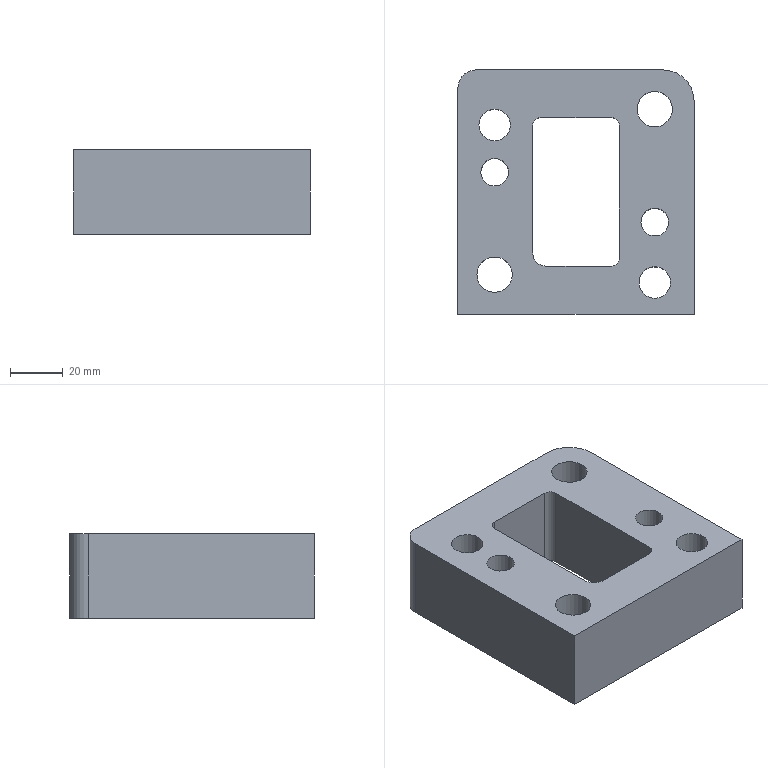Part | STEP file | lll_id3174_x_t | 1 solid | 26 faces | box 90 x 93 x 32 mm | volume 180117 mm3 | cylinder 14 | plane 12 | commonest cylinder face diameters 6 x3 10.505 x2 12 x2 13.509 x2 20.008 x2 10 x1
STEP:
#1=CARTESIAN_POINT('',(926.252,-22.25,60.5));
#2=VERTEX_POINT('',#1);
#3=CARTESIAN_POINT('',(921.,-22.25,60.5));
#4=DIRECTION('',(0.,0.,1.));
#5=DIRECTION('',(1.,0.,0.));
#6=AXIS2_PLACEMENT_3D('',#3,#4,#5);
#7=CIRCLE('',#6,5.253);
#8=EDGE_CURVE('',#2,#2,#7,.T.);
#9=ORIENTED_EDGE('',*,*,#8,.T.);
#10=EDGE_LOOP('',(#9));
#11=FACE_BOUND('',#10,.T.);
#12=CARTESIAN_POINT('',(849.996,-42.25,60.5));
#13=VERTEX_POINT('',#12);
#14=CARTESIAN_POINT('',(860.,-42.25,60.5));
#15=DIRECTION('',(0.,0.,1.));
#16=DIRECTION('',(-1.,0.,0.));
#17=AXIS2_PLACEMENT_3D('',#14,#15,#16);
#18=CIRCLE('',#17,10.004);
#19=EDGE_CURVE('',#13,#13,#18,.T.);
#20=ORIENTED_EDGE('',*,*,#19,.T.);
#21=EDGE_LOOP('',(#20));
#22=FACE_BOUND('',#21,.T.);
#23=CARTESIAN_POINT('',(874.5,14.5,60.5));
#24=VERTEX_POINT('',#23);
#25=CARTESIAN_POINT('',(874.5,-34.,60.5));
#26=VERTEX_POINT('',#25);
#27=CARTESIAN_POINT('',(874.5,0.,60.5));
#28=DIRECTION('',(0.,-1.,0.));
#29=VECTOR('',#28,1.);
#30=LINE('',#27,#29);
#31=EDGE_CURVE('',#24,#26,#30,.T.);
#32=ORIENTED_EDGE('',*,*,#31,.T.);
#33=CARTESIAN_POINT('',(879.5,-39.,60.5));
#34=VERTEX_POINT('',#33);
#35=CARTESIAN_POINT('',(879.5,-34.,60.5));
#36=DIRECTION('',(0.,0.,1.));
#37=DIRECTION('',(-1.,0.,0.));
#38=AXIS2_PLACEMENT_3D('',#35,#36,#37);
#39=CIRCLE('',#38,5.);
#40=EDGE_CURVE('',#26,#34,#39,.T.);
#41=ORIENTED_EDGE('',*,*,#40,.T.);
#42=CARTESIAN_POINT('',(904.5,-39.,60.5));
#43=VERTEX_POINT('',#42);
#44=CARTESIAN_POINT('',(891.,-39.,60.5));
#45=DIRECTION('',(1.,0.,0.));
#46=VECTOR('',#45,1.);
#47=LINE('',#44,#46);
#48=EDGE_CURVE('',#34,#43,#47,.T.);
#49=ORIENTED_EDGE('',*,*,#48,.T.);
#50=CARTESIAN_POINT('',(907.5,-36.,60.5));
#51=VERTEX_POINT('',#50);
#52=CARTESIAN_POINT('',(904.5,-36.,60.5));
#53=DIRECTION('',(0.,0.,1.));
#54=DIRECTION('',(-1.,0.,0.));
#55=AXIS2_PLACEMENT_3D('',#52,#53,#54);
#56=CIRCLE('',#55,3.);
#57=EDGE_CURVE('',#43,#51,#56,.T.);
#58=ORIENTED_EDGE('',*,*,#57,.T.);
#59=CARTESIAN_POINT('',(907.5,14.5,60.5));
#60=VERTEX_POINT('',#59);
#61=CARTESIAN_POINT('',(907.5,0.,60.5));
#62=DIRECTION('',(0.,1.,0.));
#63=VECTOR('',#62,1.);
#64=LINE('',#61,#63);
#65=EDGE_CURVE('',#51,#60,#64,.T.);
#66=ORIENTED_EDGE('',*,*,#65,.T.);
#67=CARTESIAN_POINT('',(904.5,17.5,60.5));
#68=VERTEX_POINT('',#67);
#69=CARTESIAN_POINT('',(904.5,14.5,60.5));
#70=DIRECTION('',(0.,0.,1.));
#71=DIRECTION('',(-1.,0.,0.));
#72=AXIS2_PLACEMENT_3D('',#69,#70,#71);
#73=CIRCLE('',#72,3.);
#74=EDGE_CURVE('',#60,#68,#73,.T.);
#75=ORIENTED_EDGE('',*,*,#74,.T.);
#76=CARTESIAN_POINT('',(877.5,17.5,60.5));
#77=VERTEX_POINT('',#76);
#78=CARTESIAN_POINT('',(891.,17.5,60.5));
#79=DIRECTION('',(-1.,0.,0.));
#80=VECTOR('',#79,1.);
#81=LINE('',#78,#80);
#82=EDGE_CURVE('',#68,#77,#81,.T.);
#83=ORIENTED_EDGE('',*,*,#82,.T.);
#84=CARTESIAN_POINT('',(877.5,14.5,60.5));
#85=DIRECTION('',(0.,0.,1.));
#86=DIRECTION('',(-1.,0.,0.));
#87=AXIS2_PLACEMENT_3D('',#84,#85,#86);
#88=CIRCLE('',#87,3.);
#89=EDGE_CURVE('',#77,#24,#88,.T.);
#90=ORIENTED_EDGE('',*,*,#89,.T.);
#91=EDGE_LOOP('',(#32,#41,#49,#58,#66,#75,#83,#90));
#92=FACE_BOUND('',#91,.T.);
#93=CARTESIAN_POINT('',(846.,28.75,60.5));
#94=VERTEX_POINT('',#93);
#95=CARTESIAN_POINT('',(846.,-57.25,60.5));
#96=VERTEX_POINT('',#95);
#97=CARTESIAN_POINT('',(846.,-8.25,60.5));
#98=DIRECTION('',(0.,-1.,0.));
#99=VECTOR('',#98,1.);
#100=LINE('',#97,#99);
#101=EDGE_CURVE('',#94,#96,#100,.T.);
#102=ORIENTED_EDGE('',*,*,#101,.F.);
#103=CARTESIAN_POINT('',(853.,35.75,60.5));
#104=VERTEX_POINT('',#103);
#105=CARTESIAN_POINT('',(853.,28.75,60.5));
#106=DIRECTION('',(0.,0.,-1.));
#107=DIRECTION('',(-1.,0.,0.));
#108=AXIS2_PLACEMENT_3D('',#105,#106,#107);
#109=CIRCLE('',#108,7.);
#110=EDGE_CURVE('',#94,#104,#109,.T.);
#111=ORIENTED_EDGE('',*,*,#110,.T.);
#112=CARTESIAN_POINT('',(924.,35.75,60.5));
#113=VERTEX_POINT('',#112);
#114=CARTESIAN_POINT('',(891.,35.75,60.5));
#115=DIRECTION('',(-1.,0.,0.));
#116=VECTOR('',#115,1.);
#117=LINE('',#114,#116);
#118=EDGE_CURVE('',#113,#104,#117,.T.);
#119=ORIENTED_EDGE('',*,*,#118,.F.);
#120=CARTESIAN_POINT('',(936.,23.75,60.5));
#121=VERTEX_POINT('',#120);
#122=CARTESIAN_POINT('',(924.,23.75,60.5));
#123=DIRECTION('',(0.,0.,-1.));
#124=DIRECTION('',(-1.,0.,0.));
#125=AXIS2_PLACEMENT_3D('',#122,#123,#124);
#126=CIRCLE('',#125,12.);
#127=EDGE_CURVE('',#113,#121,#126,.T.);
#128=ORIENTED_EDGE('',*,*,#127,.T.);
#129=CARTESIAN_POINT('',(936.,-57.25,60.5));
#130=VERTEX_POINT('',#129);
#131=CARTESIAN_POINT('',(936.,-8.25,60.5));
#132=DIRECTION('',(0.,1.,0.));
#133=VECTOR('',#132,1.);
#134=LINE('',#131,#133);
#135=EDGE_CURVE('',#130,#121,#134,.T.);
#136=ORIENTED_EDGE('',*,*,#135,.F.);
#137=CARTESIAN_POINT('',(891.,-57.25,60.5));
#138=DIRECTION('',(1.,0.,0.));
#139=VECTOR('',#138,1.);
#140=LINE('',#137,#139);
#141=EDGE_CURVE('',#96,#130,#140,.T.);
#142=ORIENTED_EDGE('',*,*,#141,.F.);
#143=EDGE_LOOP('',(#102,#111,#119,#128,#136,#142));
#144=FACE_BOUND('',#143,.T.);
#145=CARTESIAN_POINT('',(866.,14.75,60.5));
#146=VERTEX_POINT('',#145);
#147=CARTESIAN_POINT('',(860.,14.75,60.5));
#148=DIRECTION('',(0.,0.,-1.));
#149=DIRECTION('',(1.,0.,0.));
#150=AXIS2_PLACEMENT_3D('',#147,#148,#149);
#151=CIRCLE('',#150,6.);
#152=EDGE_CURVE('',#146,#146,#151,.T.);
#153=ORIENTED_EDGE('',*,*,#152,.F.);
#154=EDGE_LOOP('',(#153));
#155=FACE_BOUND('',#154,.T.);
#156=CARTESIAN_POINT('',(915.,-45.25,60.5));
#157=VERTEX_POINT('',#156);
#158=CARTESIAN_POINT('',(921.,-45.25,60.5));
#159=DIRECTION('',(0.,0.,-1.));
#160=DIRECTION('',(-1.,0.,0.));
#161=AXIS2_PLACEMENT_3D('',#158,#159,#160);
#162=CIRCLE('',#161,6.);
#163=EDGE_CURVE('',#157,#157,#162,.T.);
#164=ORIENTED_EDGE('',*,*,#163,.F.);
#165=EDGE_LOOP('',(#164));
#166=FACE_BOUND('',#165,.T.);
#167=CARTESIAN_POINT('',(931.004,20.75,60.5));
#168=VERTEX_POINT('',#167);
#169=CARTESIAN_POINT('',(921.,20.75,60.5));
#170=DIRECTION('',(0.,0.,1.));
#171=DIRECTION('',(1.,0.,0.));
#172=AXIS2_PLACEMENT_3D('',#169,#170,#171);
#173=CIRCLE('',#172,10.004);
#174=EDGE_CURVE('',#168,#168,#173,.T.);
#175=ORIENTED_EDGE('',*,*,#174,.T.);
#176=EDGE_LOOP('',(#175));
#177=FACE_BOUND('',#176,.T.);
#178=CARTESIAN_POINT('',(865.252,-3.25,60.5));
#179=VERTEX_POINT('',#178);
#180=CARTESIAN_POINT('',(860.,-3.25,60.5));
#181=DIRECTION('',(0.,0.,1.));
#182=DIRECTION('',(1.,0.,0.));
#183=AXIS2_PLACEMENT_3D('',#180,#181,#182);
#184=CIRCLE('',#183,5.253);
#185=EDGE_CURVE('',#179,#179,#184,.T.);
#186=ORIENTED_EDGE('',*,*,#185,.T.);
#187=EDGE_LOOP('',(#186));
#188=FACE_BOUND('',#187,.T.);
#189=CARTESIAN_POINT('',(891.,-8.25,60.5));
#190=DIRECTION('',(0.,0.,-1.));
#191=DIRECTION('',(1.,0.,0.));
#192=AXIS2_PLACEMENT_3D('',#189,#190,#191);
#193=PLANE('',#192);
#194=ADVANCED_FACE('',(#11,#22,#92,#144,#155,#166,#177,#188),#193,.T.);
#195=CARTESIAN_POINT('',(865.252,-3.25,92.5));
#196=VERTEX_POINT('',#195);
#197=CARTESIAN_POINT('',(860.,-3.25,92.5));
#198=DIRECTION('',(0.,0.,1.));
#199=DIRECTION('',(1.,0.,0.));
#200=AXIS2_PLACEMENT_3D('',#197,#198,#199);
#201=CIRCLE('',#200,5.253);
#202=EDGE_CURVE('',#196,#196,#201,.T.);
#203=ORIENTED_EDGE('',*,*,#202,.F.);
#204=EDGE_LOOP('',(#203));
#205=FACE_BOUND('',#204,.T.);
#206=CARTESIAN_POINT('',(926.252,-22.25,92.5));
#207=VERTEX_POINT('',#206);
#208=CARTESIAN_POINT('',(921.,-22.25,92.5));
#209=DIRECTION('',(0.,0.,1.));
#210=DIRECTION('',(1.,0.,0.));
#211=AXIS2_PLACEMENT_3D('',#208,#209,#210);
#212=CIRCLE('',#211,5.253);
#213=EDGE_CURVE('',#207,#207,#212,.T.);
#214=ORIENTED_EDGE('',*,*,#213,.F.);
#215=EDGE_LOOP('',(#214));
#216=FACE_BOUND('',#215,.T.);
#217=CARTESIAN_POINT('',(914.245,20.75,92.5));
#218=VERTEX_POINT('',#217);
#219=CARTESIAN_POINT('',(921.,20.75,92.5));
#220=DIRECTION('',(0.,0.,1.));
#221=DIRECTION('',(-1.,0.,0.));
#222=AXIS2_PLACEMENT_3D('',#219,#220,#221);
#223=CIRCLE('',#222,6.755);
#224=EDGE_CURVE('',#218,#218,#223,.T.);
#225=ORIENTED_EDGE('',*,*,#224,.F.);
#226=EDGE_LOOP('',(#225));
#227=FACE_BOUND('',#226,.T.);
#228=CARTESIAN_POINT('',(853.245,-42.25,92.5));
#229=VERTEX_POINT('',#228);
#230=CARTESIAN_POINT('',(860.,-42.25,92.5));
#231=DIRECTION('',(0.,0.,1.));
#232=DIRECTION('',(-1.,0.,0.));
#233=AXIS2_PLACEMENT_3D('',#230,#231,#232);
#234=CIRCLE('',#233,6.755);
#235=EDGE_CURVE('',#229,#229,#234,.T.);
#236=ORIENTED_EDGE('',*,*,#235,.F.);
#237=EDGE_LOOP('',(#236));
#238=FACE_BOUND('',#237,.T.);
#239=CARTESIAN_POINT('',(907.5,14.5,92.5));
#240=VERTEX_POINT('',#239);
#241=CARTESIAN_POINT('',(907.5,-36.,92.5));
#242=VERTEX_POINT('',#241);
#243=CARTESIAN_POINT('',(907.5,0.,92.5));
#244=DIRECTION('',(0.,-1.,0.));
#245=VECTOR('',#244,1.);
#246=LINE('',#243,#245);
#247=EDGE_CURVE('',#240,#242,#246,.T.);
#248=ORIENTED_EDGE('',*,*,#247,.T.);
#249=CARTESIAN_POINT('',(904.5,-39.,92.5));
#250=VERTEX_POINT('',#249);
#251=CARTESIAN_POINT('',(904.5,-36.,92.5));
#252=DIRECTION('',(0.,0.,-1.));
#253=DIRECTION('',(1.,0.,0.));
#254=AXIS2_PLACEMENT_3D('',#251,#252,#253);
#255=CIRCLE('',#254,3.);
#256=EDGE_CURVE('',#242,#250,#255,.T.);
#257=ORIENTED_EDGE('',*,*,#256,.T.);
#258=CARTESIAN_POINT('',(879.5,-39.,92.5));
#259=VERTEX_POINT('',#258);
#260=CARTESIAN_POINT('',(891.,-39.,92.5));
#261=DIRECTION('',(-1.,0.,0.));
#262=VECTOR('',#261,1.);
#263=LINE('',#260,#262);
#264=EDGE_CURVE('',#250,#259,#263,.T.);
#265=ORIENTED_EDGE('',*,*,#264,.T.);
#266=CARTESIAN_POINT('',(874.5,-34.,92.5));
#267=VERTEX_POINT('',#266);
#268=CARTESIAN_POINT('',(879.5,-34.,92.5));
#269=DIRECTION('',(0.,0.,-1.));
#270=DIRECTION('',(1.,0.,0.));
#271=AXIS2_PLACEMENT_3D('',#268,#269,#270);
#272=CIRCLE('',#271,5.);
#273=EDGE_CURVE('',#259,#267,#272,.T.);
#274=ORIENTED_EDGE('',*,*,#273,.T.);
#275=CARTESIAN_POINT('',(874.5,14.5,92.5));
#276=VERTEX_POINT('',#275);
#277=CARTESIAN_POINT('',(874.5,0.,92.5));
#278=DIRECTION('',(0.,1.,0.));
#279=VECTOR('',#278,1.);
#280=LINE('',#277,#279);
#281=EDGE_CURVE('',#267,#276,#280,.T.);
#282=ORIENTED_EDGE('',*,*,#281,.T.);
#283=CARTESIAN_POINT('',(877.5,17.5,92.5));
#284=VERTEX_POINT('',#283);
#285=CARTESIAN_POINT('',(877.5,14.5,92.5));
#286=DIRECTION('',(0.,0.,-1.));
#287=DIRECTION('',(1.,0.,0.));
#288=AXIS2_PLACEMENT_3D('',#285,#286,#287);
#289=CIRCLE('',#288,3.);
#290=EDGE_CURVE('',#276,#284,#289,.T.);
#291=ORIENTED_EDGE('',*,*,#290,.T.);
#292=CARTESIAN_POINT('',(904.5,17.5,92.5));
#293=VERTEX_POINT('',#292);
#294=CARTESIAN_POINT('',(891.,17.5,92.5));
#295=DIRECTION('',(1.,0.,0.));
#296=VECTOR('',#295,1.);
#297=LINE('',#294,#296);
#298=EDGE_CURVE('',#284,#293,#297,.T.);
#299=ORIENTED_EDGE('',*,*,#298,.T.);
#300=CARTESIAN_POINT('',(904.5,14.5,92.5));
#301=DIRECTION('',(0.,0.,-1.));
#302=DIRECTION('',(1.,0.,0.));
#303=AXIS2_PLACEMENT_3D('',#300,#301,#302);
#304=CIRCLE('',#303,3.);
#305=EDGE_CURVE('',#293,#240,#304,.T.);
#306=ORIENTED_EDGE('',*,*,#305,.T.);
#307=EDGE_LOOP('',(#248,#257,#265,#274,#282,#291,#299,#306));
#308=FACE_BOUND('',#307,.T.);
#309=CARTESIAN_POINT('',(853.,35.75,92.5));
#310=VERTEX_POINT('',#309);
#311=CARTESIAN_POINT('',(924.,35.75,92.5));
#312=VERTEX_POINT('',#311);
#313=CARTESIAN_POINT('',(891.,35.75,92.5));
#314=DIRECTION('',(1.,0.,0.));
#315=VECTOR('',#314,1.);
#316=LINE('',#313,#315);
#317=EDGE_CURVE('',#310,#312,#316,.T.);
#318=ORIENTED_EDGE('',*,*,#317,.F.);
#319=CARTESIAN_POINT('',(846.,28.75,92.5));
#320=VERTEX_POINT('',#319);
#321=CARTESIAN_POINT('',(853.,28.75,92.5));
#322=DIRECTION('',(0.,0.,1.));
#323=DIRECTION('',(1.,0.,0.));
#324=AXIS2_PLACEMENT_3D('',#321,#322,#323);
#325=CIRCLE('',#324,7.);
#326=EDGE_CURVE('',#310,#320,#325,.T.);
#327=ORIENTED_EDGE('',*,*,#326,.T.);
#328=CARTESIAN_POINT('',(846.,-57.25,92.5));
#329=VERTEX_POINT('',#328);
#330=CARTESIAN_POINT('',(846.,-8.25,92.5));
#331=DIRECTION('',(0.,1.,0.));
#332=VECTOR('',#331,1.);
#333=LINE('',#330,#332);
#334=EDGE_CURVE('',#329,#320,#333,.T.);
#335=ORIENTED_EDGE('',*,*,#334,.F.);
#336=CARTESIAN_POINT('',(936.,-57.25,92.5));
#337=VERTEX_POINT('',#336);
#338=CARTESIAN_POINT('',(891.,-57.25,92.5));
#339=DIRECTION('',(-1.,0.,0.));
#340=VECTOR('',#339,1.);
#341=LINE('',#338,#340);
#342=EDGE_CURVE('',#337,#329,#341,.T.);
#343=ORIENTED_EDGE('',*,*,#342,.F.);
#344=CARTESIAN_POINT('',(936.,23.75,92.5));
#345=VERTEX_POINT('',#344);
#346=CARTESIAN_POINT('',(936.,-8.25,92.5));
#347=DIRECTION('',(0.,-1.,0.));
#348=VECTOR('',#347,1.);
#349=LINE('',#346,#348);
#350=EDGE_CURVE('',#345,#337,#349,.T.);
#351=ORIENTED_EDGE('',*,*,#350,.F.);
#352=CARTESIAN_POINT('',(924.,23.75,92.5));
#353=DIRECTION('',(0.,0.,1.));
#354=DIRECTION('',(1.,0.,0.));
#355=AXIS2_PLACEMENT_3D('',#352,#353,#354);
#356=CIRCLE('',#355,12.);
#357=EDGE_CURVE('',#345,#312,#356,.T.);
#358=ORIENTED_EDGE('',*,*,#357,.T.);
#359=EDGE_LOOP('',(#318,#327,#335,#343,#351,#358));
#360=FACE_BOUND('',#359,.T.);
#361=CARTESIAN_POINT('',(854.,14.75,92.5));
#362=VERTEX_POINT('',#361);
#363=CARTESIAN_POINT('',(860.,14.75,92.5));
#364=DIRECTION('',(0.,0.,-1.));
#365=DIRECTION('',(-1.,0.,0.));
#366=AXIS2_PLACEMENT_3D('',#363,#364,#365);
#367=CIRCLE('',#366,6.);
#368=EDGE_CURVE('',#362,#362,#367,.T.);
#369=ORIENTED_EDGE('',*,*,#368,.T.);
#370=EDGE_LOOP('',(#369));
#371=FACE_BOUND('',#370,.T.);
#372=CARTESIAN_POINT('',(927.,-45.25,92.5));
#373=VERTEX_POINT('',#372);
#374=CARTESIAN_POINT('',(921.,-45.25,92.5));
#375=DIRECTION('',(0.,0.,-1.));
#376=DIRECTION('',(1.,0.,0.));
#377=AXIS2_PLACEMENT_3D('',#374,#375,#376);
#378=CIRCLE('',#377,6.);
#379=EDGE_CURVE('',#373,#373,#378,.T.);
#380=ORIENTED_EDGE('',*,*,#379,.T.);
#381=EDGE_LOOP('',(#380));
#382=FACE_BOUND('',#381,.T.);
#383=CARTESIAN_POINT('',(891.,-8.25,92.5));
#384=DIRECTION('',(0.,0.,1.));
#385=DIRECTION('',(-1.,0.,0.));
#386=AXIS2_PLACEMENT_3D('',#383,#384,#385);
#387=PLANE('',#386);
#388=ADVANCED_FACE('',(#205,#216,#227,#238,#308,#360,#371,#382),#387,.T.);
#389=ORIENTED_EDGE('',*,*,#118,.T.);
#390=CARTESIAN_POINT('',(853.,35.75,60.5));
#391=DIRECTION('',(0.,0.,1.));
#392=VECTOR('',#391,1.);
#393=LINE('',#390,#392);
#394=EDGE_CURVE('',#104,#310,#393,.T.);
#395=ORIENTED_EDGE('',*,*,#394,.T.);
#396=ORIENTED_EDGE('',*,*,#317,.T.);
#397=CARTESIAN_POINT('',(924.,35.75,60.5));
#398=DIRECTION('',(0.,0.,-1.));
#399=VECTOR('',#398,1.);
#400=LINE('',#397,#399);
#401=EDGE_CURVE('',#312,#113,#400,.T.);
#402=ORIENTED_EDGE('',*,*,#401,.T.);
#403=EDGE_LOOP('',(#389,#395,#396,#402));
#404=FACE_OUTER_BOUND('',#403,.T.);
#405=CARTESIAN_POINT('',(891.,35.75,60.5));
#406=DIRECTION('',(0.,1.,0.));
#407=DIRECTION('',(0.,0.,-1.));
#408=AXIS2_PLACEMENT_3D('',#405,#406,#407);
#409=PLANE('',#408);
#410=ADVANCED_FACE('',(#404),#409,.T.);
#411=ORIENTED_EDGE('',*,*,#135,.T.);
#412=CARTESIAN_POINT('',(936.,23.75,60.5));
#413=DIRECTION('',(0.,0.,1.));
#414=VECTOR('',#413,1.);
#415=LINE('',#412,#414);
#416=EDGE_CURVE('',#121,#345,#415,.T.);
#417=ORIENTED_EDGE('',*,*,#416,.T.);
#418=ORIENTED_EDGE('',*,*,#350,.T.);
#419=CARTESIAN_POINT('',(936.,-57.25,60.5));
#420=DIRECTION('',(0.,0.,1.));
#421=VECTOR('',#420,1.);
#422=LINE('',#419,#421);
#423=EDGE_CURVE('',#130,#337,#422,.T.);
#424=ORIENTED_EDGE('',*,*,#423,.F.);
#425=EDGE_LOOP('',(#411,#417,#418,#424));
#426=FACE_OUTER_BOUND('',#425,.T.);
#427=CARTESIAN_POINT('',(936.,-8.25,60.5));
#428=DIRECTION('',(1.,0.,0.));
#429=DIRECTION('',(0.,0.,1.));
#430=AXIS2_PLACEMENT_3D('',#427,#428,#429);
#431=PLANE('',#430);
#432=ADVANCED_FACE('',(#426),#431,.T.);
#433=ORIENTED_EDGE('',*,*,#423,.T.);
#434=ORIENTED_EDGE('',*,*,#342,.T.);
#435=CARTESIAN_POINT('',(846.,-57.25,60.5));
#436=DIRECTION('',(0.,0.,1.));
#437=VECTOR('',#436,1.);
#438=LINE('',#435,#437);
#439=EDGE_CURVE('',#96,#329,#438,.T.);
#440=ORIENTED_EDGE('',*,*,#439,.F.);
#441=ORIENTED_EDGE('',*,*,#141,.T.);
#442=EDGE_LOOP('',(#433,#434,#440,#441));
#443=FACE_OUTER_BOUND('',#442,.T.);
#444=CARTESIAN_POINT('',(891.,-57.25,60.5));
#445=DIRECTION('',(0.,-1.,0.));
#446=DIRECTION('',(0.,0.,1.));
#447=AXIS2_PLACEMENT_3D('',#444,#445,#446);
#448=PLANE('',#447);
#449=ADVANCED_FACE('',(#443),#448,.T.);
#450=ORIENTED_EDGE('',*,*,#334,.T.);
#451=CARTESIAN_POINT('',(846.,28.75,60.5));
#452=DIRECTION('',(0.,0.,-1.));
#453=VECTOR('',#452,1.);
#454=LINE('',#451,#453);
#455=EDGE_CURVE('',#320,#94,#454,.T.);
#456=ORIENTED_EDGE('',*,*,#455,.T.);
#457=ORIENTED_EDGE('',*,*,#101,.T.);
#458=ORIENTED_EDGE('',*,*,#439,.T.);
#459=EDGE_LOOP('',(#450,#456,#457,#458));
#460=FACE_OUTER_BOUND('',#459,.T.);
#461=CARTESIAN_POINT('',(846.,-8.25,60.5));
#462=DIRECTION('',(-1.,0.,0.));
#463=DIRECTION('',(0.,0.,-1.));
#464=AXIS2_PLACEMENT_3D('',#461,#462,#463);
#465=PLANE('',#464);
#466=ADVANCED_FACE('',(#460),#465,.T.);
#467=ORIENTED_EDGE('',*,*,#65,.F.);
#468=CARTESIAN_POINT('',(907.5,-36.,92.5));
#469=DIRECTION('',(0.,0.,1.));
#470=VECTOR('',#469,1.);
#471=LINE('',#468,#470);
#472=EDGE_CURVE('',#51,#242,#471,.T.);
#473=ORIENTED_EDGE('',*,*,#472,.T.);
#474=ORIENTED_EDGE('',*,*,#247,.F.);
#475=CARTESIAN_POINT('',(907.5,14.5,60.5));
#476=DIRECTION('',(0.,0.,-1.));
#477=VECTOR('',#476,1.);
#478=LINE('',#475,#477);
#479=EDGE_CURVE('',#240,#60,#478,.T.);
#480=ORIENTED_EDGE('',*,*,#479,.T.);
#481=EDGE_LOOP('',(#467,#473,#474,#480));
#482=FACE_OUTER_BOUND('',#481,.T.);
#483=CARTESIAN_POINT('',(907.5,0.,-8.5));
#484=DIRECTION('',(1.,0.,0.));
#485=DIRECTION('',(0.,0.,1.));
#486=AXIS2_PLACEMENT_3D('',#483,#484,#485);
#487=PLANE('',#486);
#488=ADVANCED_FACE('',(#482),#487,.F.);
#489=ORIENTED_EDGE('',*,*,#48,.F.);
#490=CARTESIAN_POINT('',(879.5,-39.,92.5));
#491=DIRECTION('',(0.,0.,1.));
#492=VECTOR('',#491,1.);
#493=LINE('',#490,#492);
#494=EDGE_CURVE('',#34,#259,#493,.T.);
#495=ORIENTED_EDGE('',*,*,#494,.T.);
#496=ORIENTED_EDGE('',*,*,#264,.F.);
#497=CARTESIAN_POINT('',(904.5,-39.,60.5));
#498=DIRECTION('',(0.,0.,-1.));
#499=VECTOR('',#498,1.);
#500=LINE('',#497,#499);
#501=EDGE_CURVE('',#250,#43,#500,.T.);
#502=ORIENTED_EDGE('',*,*,#501,.T.);
#503=EDGE_LOOP('',(#489,#495,#496,#502));
#504=FACE_OUTER_BOUND('',#503,.T.);
#505=CARTESIAN_POINT('',(891.,-39.,-8.5));
#506=DIRECTION('',(0.,-1.,0.));
#507=DIRECTION('',(0.,0.,1.));
#508=AXIS2_PLACEMENT_3D('',#505,#506,#507);
#509=PLANE('',#508);
#510=ADVANCED_FACE('',(#504),#509,.F.);
#511=ORIENTED_EDGE('',*,*,#281,.F.);
#512=CARTESIAN_POINT('',(874.5,-34.,60.5));
#513=DIRECTION('',(0.,0.,-1.));
#514=VECTOR('',#513,1.);
#515=LINE('',#512,#514);
#516=EDGE_CURVE('',#267,#26,#515,.T.);
#517=ORIENTED_EDGE('',*,*,#516,.T.);
#518=ORIENTED_EDGE('',*,*,#31,.F.);
#519=CARTESIAN_POINT('',(874.5,14.5,92.5));
#520=DIRECTION('',(0.,0.,1.));
#521=VECTOR('',#520,1.);
#522=LINE('',#519,#521);
#523=EDGE_CURVE('',#24,#276,#522,.T.);
#524=ORIENTED_EDGE('',*,*,#523,.T.);
#525=EDGE_LOOP('',(#511,#517,#518,#524));
#526=FACE_OUTER_BOUND('',#525,.T.);
#527=CARTESIAN_POINT('',(874.5,0.,-8.5));
#528=DIRECTION('',(-1.,0.,0.));
#529=DIRECTION('',(0.,0.,-1.));
#530=AXIS2_PLACEMENT_3D('',#527,#528,#529);
#531=PLANE('',#530);
#532=ADVANCED_FACE('',(#526),#531,.F.);
#533=ORIENTED_EDGE('',*,*,#82,.F.);
#534=CARTESIAN_POINT('',(904.5,17.5,92.5));
#535=DIRECTION('',(0.,0.,1.));
#536=VECTOR('',#535,1.);
#537=LINE('',#534,#536);
#538=EDGE_CURVE('',#68,#293,#537,.T.);
#539=ORIENTED_EDGE('',*,*,#538,.T.);
#540=ORIENTED_EDGE('',*,*,#298,.F.);
#541=CARTESIAN_POINT('',(877.5,17.5,60.5));
#542=DIRECTION('',(0.,0.,-1.));
#543=VECTOR('',#542,1.);
#544=LINE('',#541,#543);
#545=EDGE_CURVE('',#284,#77,#544,.T.);
#546=ORIENTED_EDGE('',*,*,#545,.T.);
#547=EDGE_LOOP('',(#533,#539,#540,#546));
#548=FACE_OUTER_BOUND('',#547,.T.);
#549=CARTESIAN_POINT('',(891.,17.5,-8.5));
#550=DIRECTION('',(0.,1.,0.));
#551=DIRECTION('',(0.,0.,-1.));
#552=AXIS2_PLACEMENT_3D('',#549,#550,#551);
#553=PLANE('',#552);
#554=ADVANCED_FACE('',(#548),#553,.F.);
#555=CARTESIAN_POINT('',(849.996,-42.25,75.5));
#556=VERTEX_POINT('',#555);
#557=CARTESIAN_POINT('',(860.,-42.25,75.5));
#558=DIRECTION('',(0.,0.,1.));
#559=DIRECTION('',(-1.,0.,0.));
#560=AXIS2_PLACEMENT_3D('',#557,#558,#559);
#561=CIRCLE('',#560,10.004);
#562=EDGE_CURVE('',#556,#556,#561,.T.);
#563=ORIENTED_EDGE('',*,*,#562,.T.);
#564=EDGE_LOOP('',(#563));
#565=FACE_BOUND('',#564,.T.);
#566=ORIENTED_EDGE('',*,*,#19,.F.);
#567=EDGE_LOOP('',(#566));
#568=FACE_BOUND('',#567,.T.);
#569=CARTESIAN_POINT('',(860.,-42.25,60.5));
#570=DIRECTION('',(0.,0.,1.));
#571=DIRECTION('',(-1.,0.,0.));
#572=AXIS2_PLACEMENT_3D('',#569,#570,#571);
#573=CYLINDRICAL_SURFACE('',#572,10.004);
#574=ADVANCED_FACE('',(#565,#568),#573,.F.);
#575=ORIENTED_EDGE('',*,*,#235,.T.);
#576=EDGE_LOOP('',(#575));
#577=FACE_BOUND('',#576,.T.);
#578=CARTESIAN_POINT('',(853.245,-42.25,75.5));
#579=VERTEX_POINT('',#578);
#580=CARTESIAN_POINT('',(860.,-42.25,75.5));
#581=DIRECTION('',(0.,0.,1.));
#582=DIRECTION('',(-1.,0.,0.));
#583=AXIS2_PLACEMENT_3D('',#580,#581,#582);
#584=CIRCLE('',#583,6.755);
#585=EDGE_CURVE('',#579,#579,#584,.T.);
#586=ORIENTED_EDGE('',*,*,#585,.F.);
#587=EDGE_LOOP('',(#586));
#588=FACE_BOUND('',#587,.T.);
#589=CARTESIAN_POINT('',(860.,-42.25,57.5));
#590=DIRECTION('',(0.,0.,1.));
#591=DIRECTION('',(-1.,0.,0.));
#592=AXIS2_PLACEMENT_3D('',#589,#590,#591);
#593=CYLINDRICAL_SURFACE('',#592,6.755);
#594=ADVANCED_FACE('',(#577,#588),#593,.F.);
#595=ORIENTED_EDGE('',*,*,#585,.T.);
#596=EDGE_LOOP('',(#595));
#597=FACE_BOUND('',#596,.T.);
#598=ORIENTED_EDGE('',*,*,#562,.F.);
#599=EDGE_LOOP('',(#598));
#600=FACE_BOUND('',#599,.T.);
#601=CARTESIAN_POINT('',(860.,-37.25,75.5));
#602=DIRECTION('',(0.,0.,1.));
#603=DIRECTION('',(-1.,0.,0.));
#604=AXIS2_PLACEMENT_3D('',#601,#602,#603);
#605=PLANE('',#604);
#606=ADVANCED_FACE('',(#597,#600),#605,.F.);
#607=ORIENTED_EDGE('',*,*,#152,.T.);
#608=EDGE_LOOP('',(#607));
#609=FACE_BOUND('',#608,.T.);
#610=ORIENTED_EDGE('',*,*,#368,.F.);
#611=EDGE_LOOP('',(#610));
#612=FACE_BOUND('',#611,.T.);
#613=CARTESIAN_POINT('',(860.,14.75,57.5));
#614=DIRECTION('',(0.,0.,1.));
#615=DIRECTION('',(-1.,0.,0.));
#616=AXIS2_PLACEMENT_3D('',#613,#614,#615);
#617=CYLINDRICAL_SURFACE('',#616,6.);
#618=ADVANCED_FACE('',(#609,#612),#617,.F.);
#619=ORIENTED_EDGE('',*,*,#163,.T.);
#620=EDGE_LOOP('',(#619));
#621=FACE_BOUND('',#620,.T.);
#622=ORIENTED_EDGE('',*,*,#379,.F.);
#623=EDGE_LOOP('',(#622));
#624=FACE_BOUND('',#623,.T.);
#625=CARTESIAN_POINT('',(921.,-45.25,57.5));
#626=DIRECTION('',(0.,0.,1.));
#627=DIRECTION('',(1.,0.,0.));
#628=AXIS2_PLACEMENT_3D('',#625,#626,#627);
#629=CYLINDRICAL_SURFACE('',#628,6.);
#630=ADVANCED_FACE('',(#621,#624),#629,.F.);
#631=CARTESIAN_POINT('',(931.004,20.75,75.5));
#632=VERTEX_POINT('',#631);
#633=CARTESIAN_POINT('',(921.,20.75,75.5));
#634=DIRECTION('',(0.,0.,1.));
#635=DIRECTION('',(1.,0.,0.));
#636=AXIS2_PLACEMENT_3D('',#633,#634,#635);
#637=CIRCLE('',#636,10.004);
#638=EDGE_CURVE('',#632,#632,#637,.T.);
#639=ORIENTED_EDGE('',*,*,#638,.T.);
#640=EDGE_LOOP('',(#639));
#641=FACE_BOUND('',#640,.T.);
#642=ORIENTED_EDGE('',*,*,#174,.F.);
#643=EDGE_LOOP('',(#642));
#644=FACE_BOUND('',#643,.T.);
#645=CARTESIAN_POINT('',(921.,20.75,60.5));
#646=DIRECTION('',(0.,0.,1.));
#647=DIRECTION('',(1.,0.,0.));
#648=AXIS2_PLACEMENT_3D('',#645,#646,#647);
#649=CYLINDRICAL_SURFACE('',#648,10.004);
#650=ADVANCED_FACE('',(#641,#644),#649,.F.);
#651=ORIENTED_EDGE('',*,*,#224,.T.);
#652=EDGE_LOOP('',(#651));
#653=FACE_BOUND('',#652,.T.);
#654=CARTESIAN_POINT('',(927.754,20.75,75.5));
#655=VERTEX_POINT('',#654);
#656=CARTESIAN_POINT('',(921.,20.75,75.5));
#657=DIRECTION('',(0.,0.,1.));
#658=DIRECTION('',(1.,0.,0.));
#659=AXIS2_PLACEMENT_3D('',#656,#657,#658);
#660=CIRCLE('',#659,6.755);
#661=EDGE_CURVE('',#655,#655,#660,.T.);
#662=ORIENTED_EDGE('',*,*,#661,.F.);
#663=EDGE_LOOP('',(#662));
#664=FACE_BOUND('',#663,.T.);
#665=CARTESIAN_POINT('',(921.,20.75,57.5));
#666=DIRECTION('',(0.,0.,1.));
#667=DIRECTION('',(1.,0.,0.));
#668=AXIS2_PLACEMENT_3D('',#665,#666,#667);
#669=CYLINDRICAL_SURFACE('',#668,6.755);
#670=ADVANCED_FACE('',(#653,#664),#669,.F.);
#671=ORIENTED_EDGE('',*,*,#661,.T.);
#672=EDGE_LOOP('',(#671));
#673=FACE_BOUND('',#672,.T.);
#674=ORIENTED_EDGE('',*,*,#638,.F.);
#675=EDGE_LOOP('',(#674));
#676=FACE_BOUND('',#675,.T.);
#677=CARTESIAN_POINT('',(921.,20.75,75.5));
#678=DIRECTION('',(0.,0.,1.));
#679=DIRECTION('',(1.,0.,0.));
#680=AXIS2_PLACEMENT_3D('',#677,#678,#679);
#681=PLANE('',#680);
#682=ADVANCED_FACE('',(#673,#676),#681,.F.);
#683=ORIENTED_EDGE('',*,*,#74,.F.);
#684=ORIENTED_EDGE('',*,*,#479,.F.);
#685=ORIENTED_EDGE('',*,*,#305,.F.);
#686=ORIENTED_EDGE('',*,*,#538,.F.);
#687=EDGE_LOOP('',(#683,#684,#685,#686));
#688=FACE_OUTER_BOUND('',#687,.T.);
#689=CARTESIAN_POINT('',(904.5,14.5,-8.5));
#690=DIRECTION('',(0.,0.,-1.));
#691=DIRECTION('',(-1.,0.,0.));
#692=AXIS2_PLACEMENT_3D('',#689,#690,#691);
#693=CYLINDRICAL_SURFACE('',#692,3.);
#694=ADVANCED_FACE('',(#688),#693,.F.);
#695=ORIENTED_EDGE('',*,*,#89,.F.);
#696=ORIENTED_EDGE('',*,*,#545,.F.);
#697=ORIENTED_EDGE('',*,*,#290,.F.);
#698=ORIENTED_EDGE('',*,*,#523,.F.);
#699=EDGE_LOOP('',(#695,#696,#697,#698));
#700=FACE_OUTER_BOUND('',#699,.T.);
#701=CARTESIAN_POINT('',(877.5,14.5,-8.5));
#702=DIRECTION('',(0.,0.,-1.));
#703=DIRECTION('',(-1.,0.,0.));
#704=AXIS2_PLACEMENT_3D('',#701,#702,#703);
#705=CYLINDRICAL_SURFACE('',#704,3.);
#706=ADVANCED_FACE('',(#700),#705,.F.);
#707=ORIENTED_EDGE('',*,*,#256,.F.);
#708=ORIENTED_EDGE('',*,*,#472,.F.);
#709=ORIENTED_EDGE('',*,*,#57,.F.);
#710=ORIENTED_EDGE('',*,*,#501,.F.);
#711=EDGE_LOOP('',(#707,#708,#709,#710));
#712=FACE_OUTER_BOUND('',#711,.T.);
#713=CARTESIAN_POINT('',(904.5,-36.,-8.5));
#714=DIRECTION('',(0.,0.,1.));
#715=DIRECTION('',(1.,0.,0.));
#716=AXIS2_PLACEMENT_3D('',#713,#714,#715);
#717=CYLINDRICAL_SURFACE('',#716,3.);
#718=ADVANCED_FACE('',(#712),#717,.F.);
#719=ORIENTED_EDGE('',*,*,#273,.F.);
#720=ORIENTED_EDGE('',*,*,#494,.F.);
#721=ORIENTED_EDGE('',*,*,#40,.F.);
#722=ORIENTED_EDGE('',*,*,#516,.F.);
#723=EDGE_LOOP('',(#719,#720,#721,#722));
#724=FACE_OUTER_BOUND('',#723,.T.);
#725=CARTESIAN_POINT('',(879.5,-34.,-8.5));
#726=DIRECTION('',(0.,0.,1.));
#727=DIRECTION('',(1.,0.,0.));
#728=AXIS2_PLACEMENT_3D('',#725,#726,#727);
#729=CYLINDRICAL_SURFACE('',#728,5.);
#730=ADVANCED_FACE('',(#724),#729,.F.);
#731=ORIENTED_EDGE('',*,*,#213,.T.);
#732=EDGE_LOOP('',(#731));
#733=FACE_BOUND('',#732,.T.);
#734=ORIENTED_EDGE('',*,*,#8,.F.);
#735=EDGE_LOOP('',(#734));
#736=FACE_BOUND('',#735,.T.);
#737=CARTESIAN_POINT('',(921.,-22.25,60.5));
#738=DIRECTION('',(0.,0.,1.));
#739=DIRECTION('',(1.,0.,0.));
#740=AXIS2_PLACEMENT_3D('',#737,#738,#739);
#741=CYLINDRICAL_SURFACE('',#740,5.253);
#742=ADVANCED_FACE('',(#733,#736),#741,.F.);
#743=ORIENTED_EDGE('',*,*,#202,.T.);
#744=EDGE_LOOP('',(#743));
#745=FACE_BOUND('',#744,.T.);
#746=ORIENTED_EDGE('',*,*,#185,.F.);
#747=EDGE_LOOP('',(#746));
#748=FACE_BOUND('',#747,.T.);
#749=CARTESIAN_POINT('',(860.,-3.25,60.5));
#750=DIRECTION('',(0.,0.,1.));
#751=DIRECTION('',(1.,0.,0.));
#752=AXIS2_PLACEMENT_3D('',#749,#750,#751);
#753=CYLINDRICAL_SURFACE('',#752,5.253);
#754=ADVANCED_FACE('',(#745,#748),#753,.F.);
#755=ORIENTED_EDGE('',*,*,#127,.F.);
#756=ORIENTED_EDGE('',*,*,#401,.F.);
#757=ORIENTED_EDGE('',*,*,#357,.F.);
#758=ORIENTED_EDGE('',*,*,#416,.F.);
#759=EDGE_LOOP('',(#755,#756,#757,#758));
#760=FACE_OUTER_BOUND('',#759,.T.);
#761=CARTESIAN_POINT('',(924.,23.75,60.5));
#762=DIRECTION('',(0.,0.,1.));
#763=DIRECTION('',(1.,0.,0.));
#764=AXIS2_PLACEMENT_3D('',#761,#762,#763);
#765=CYLINDRICAL_SURFACE('',#764,12.);
#766=ADVANCED_FACE('',(#760),#765,.T.);
#767=ORIENTED_EDGE('',*,*,#110,.F.);
#768=ORIENTED_EDGE('',*,*,#455,.F.);
#769=ORIENTED_EDGE('',*,*,#326,.F.);
#770=ORIENTED_EDGE('',*,*,#394,.F.);
#771=EDGE_LOOP('',(#767,#768,#769,#770));
#772=FACE_OUTER_BOUND('',#771,.T.);
#773=CARTESIAN_POINT('',(853.,28.75,60.5));
#774=DIRECTION('',(0.,0.,1.));
#775=DIRECTION('',(1.,0.,0.));
#776=AXIS2_PLACEMENT_3D('',#773,#774,#775);
#777=CYLINDRICAL_SURFACE('',#776,7.);
#778=ADVANCED_FACE('',(#772),#777,.T.);
#779=CLOSED_SHELL('',(#194,#388,#410,#432,#449,#466,#488,#510,#532,#554,#574,#594,#606,#618,#630,#650,#670,#682,#694,#706,#718,#730,#742,#754,#766,#778));
#780=MANIFOLD_SOLID_BREP('',#779);
#781=(LENGTH_UNIT()NAMED_UNIT(*)SI_UNIT(.MILLI.,.METRE.));
#782=UNCERTAINTY_MEASURE_WITH_UNIT(LENGTH_MEASURE(0.00002),#781,'','');
#783=(NAMED_UNIT(*)PLANE_ANGLE_UNIT()SI_UNIT($,.RADIAN.));
#784=PLANE_ANGLE_MEASURE_WITH_UNIT(PLANE_ANGLE_MEASURE(0.01745),#783);
#785=DIMENSIONAL_EXPONENTS(0.,0.,0.,0.,0.,0.,0.);
#786=(CONVERSION_BASED_UNIT('DEGREE',#784)NAMED_UNIT(#785)PLANE_ANGLE_UNIT());
#787=(NAMED_UNIT(*)SI_UNIT($,.STERADIAN.)SOLID_ANGLE_UNIT());
#788=(GEOMETRIC_REPRESENTATION_CONTEXT(3)GLOBAL_UNCERTAINTY_ASSIGNED_CONTEXT((#782))GLOBAL_UNIT_ASSIGNED_CONTEXT((#781,#786,#787))REPRESENTATION_CONTEXT('',''));
#789=ADVANCED_BREP_SHAPE_REPRESENTATION('',(#780),#788);